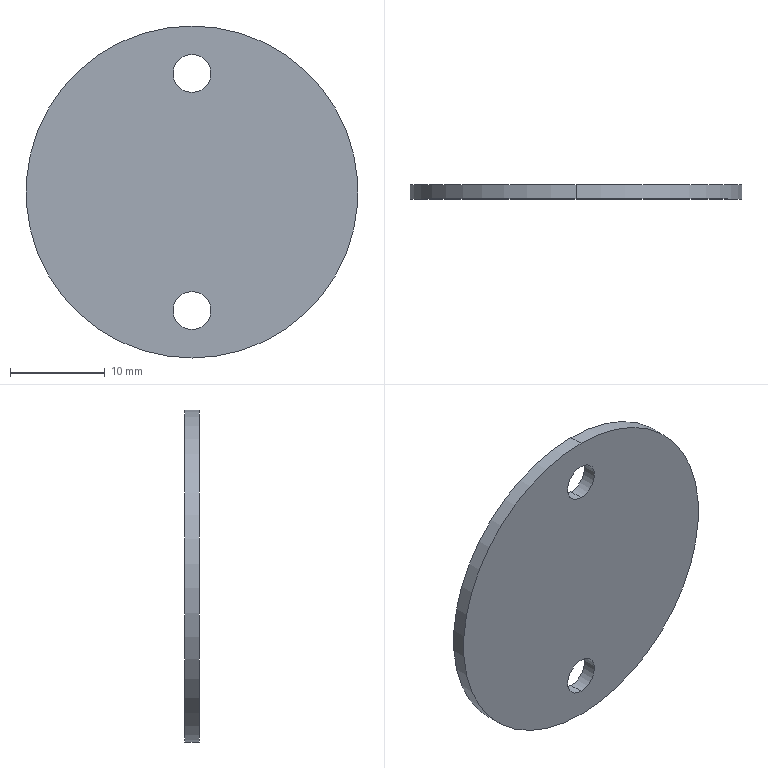Part | STEP file | 1519D1-4.stp.STEP | 1 solid | 8 faces | box 35 x 1.5 x 35 mm | volume 1405 mm3 | cylinder 6 | plane 2 | commonest cylinder face diameters 4 x4 35 x2
STEP:
#1=CARTESIAN_POINT('',(0.,0.,14.5));
#2=VERTEX_POINT('',#1);
#3=CARTESIAN_POINT('',(0.,0.,10.5));
#4=VERTEX_POINT('',#3);
#5=CARTESIAN_POINT('',(0.,0.,12.5));
#6=DIRECTION('',(0.,1.,0.));
#7=DIRECTION('',(0.,0.,1.));
#8=AXIS2_PLACEMENT_3D('',#5,#6,#7);
#9=CIRCLE('',#8,2.);
#10=EDGE_CURVE('',#2,#4,#9,.T.);
#11=ORIENTED_EDGE('',*,*,#10,.T.);
#12=CARTESIAN_POINT('',(0.,0.,12.5));
#13=DIRECTION('',(0.,1.,0.));
#14=DIRECTION('',(0.,0.,-1.));
#15=AXIS2_PLACEMENT_3D('',#12,#13,#14);
#16=CIRCLE('',#15,2.);
#17=EDGE_CURVE('',#4,#2,#16,.T.);
#18=ORIENTED_EDGE('',*,*,#17,.T.);
#19=EDGE_LOOP('',(#11,#18));
#20=FACE_BOUND('',#19,.T.);
#21=CARTESIAN_POINT('',(0.,0.,-10.5));
#22=VERTEX_POINT('',#21);
#23=CARTESIAN_POINT('',(0.,0.,-14.5));
#24=VERTEX_POINT('',#23);
#25=CARTESIAN_POINT('',(0.,0.,-12.5));
#26=DIRECTION('',(0.,1.,0.));
#27=DIRECTION('',(0.,0.,1.));
#28=AXIS2_PLACEMENT_3D('',#25,#26,#27);
#29=CIRCLE('',#28,2.);
#30=EDGE_CURVE('',#22,#24,#29,.T.);
#31=ORIENTED_EDGE('',*,*,#30,.T.);
#32=CARTESIAN_POINT('',(0.,0.,-12.5));
#33=DIRECTION('',(0.,1.,0.));
#34=DIRECTION('',(0.,0.,-1.));
#35=AXIS2_PLACEMENT_3D('',#32,#33,#34);
#36=CIRCLE('',#35,2.);
#37=EDGE_CURVE('',#24,#22,#36,.T.);
#38=ORIENTED_EDGE('',*,*,#37,.T.);
#39=EDGE_LOOP('',(#31,#38));
#40=FACE_BOUND('',#39,.T.);
#41=CARTESIAN_POINT('',(0.,0.,17.5));
#42=VERTEX_POINT('',#41);
#43=CARTESIAN_POINT('',(0.,0.,-17.5));
#44=VERTEX_POINT('',#43);
#45=CARTESIAN_POINT('',(0.,0.,0.));
#46=DIRECTION('',(0.,1.,0.));
#47=DIRECTION('',(0.,0.,1.));
#48=AXIS2_PLACEMENT_3D('',#45,#46,#47);
#49=CIRCLE('',#48,17.5);
#50=EDGE_CURVE('',#42,#44,#49,.T.);
#51=ORIENTED_EDGE('',*,*,#50,.F.);
#52=CARTESIAN_POINT('',(0.,0.,0.));
#53=DIRECTION('',(0.,1.,0.));
#54=DIRECTION('',(0.,0.,-1.));
#55=AXIS2_PLACEMENT_3D('',#52,#53,#54);
#56=CIRCLE('',#55,17.5);
#57=EDGE_CURVE('',#44,#42,#56,.T.);
#58=ORIENTED_EDGE('',*,*,#57,.F.);
#59=EDGE_LOOP('',(#51,#58));
#60=FACE_OUTER_BOUND('',#59,.T.);
#61=CARTESIAN_POINT('',(0.,0.,0.));
#62=DIRECTION('',(0.,1.,0.));
#63=DIRECTION('',(1.,0.,0.));
#64=AXIS2_PLACEMENT_3D('',#61,#62,#63);
#65=PLANE('',#64);
#66=ADVANCED_FACE('',(#20,#40,#60),#65,.F.);
#67=CARTESIAN_POINT('',(0.,1.5,17.5));
#68=VERTEX_POINT('',#67);
#69=CARTESIAN_POINT('',(0.,0.,17.5));
#70=DIRECTION('',(0.,1.,0.));
#71=VECTOR('',#70,1000.);
#72=LINE('',#69,#71);
#73=EDGE_CURVE('',#42,#68,#72,.T.);
#74=ORIENTED_EDGE('',*,*,#73,.T.);
#75=CARTESIAN_POINT('',(0.,1.5,-17.5));
#76=VERTEX_POINT('',#75);
#77=CARTESIAN_POINT('',(0.,1.5,0.));
#78=DIRECTION('',(0.,1.,0.));
#79=DIRECTION('',(0.,0.,-1.));
#80=AXIS2_PLACEMENT_3D('',#77,#78,#79);
#81=CIRCLE('',#80,17.5);
#82=EDGE_CURVE('',#76,#68,#81,.T.);
#83=ORIENTED_EDGE('',*,*,#82,.F.);
#84=CARTESIAN_POINT('',(0.,0.,-17.5));
#85=DIRECTION('',(0.,1.,0.));
#86=VECTOR('',#85,1000.);
#87=LINE('',#84,#86);
#88=EDGE_CURVE('',#44,#76,#87,.T.);
#89=ORIENTED_EDGE('',*,*,#88,.F.);
#90=ORIENTED_EDGE('',*,*,#57,.T.);
#91=EDGE_LOOP('',(#74,#83,#89,#90));
#92=FACE_OUTER_BOUND('',#91,.T.);
#93=CARTESIAN_POINT('',(0.,0.,0.));
#94=DIRECTION('',(0.,1.,0.));
#95=DIRECTION('',(0.,0.,-1.));
#96=AXIS2_PLACEMENT_3D('',#93,#94,#95);
#97=CYLINDRICAL_SURFACE('',#96,17.5);
#98=ADVANCED_FACE('',(#92),#97,.T.);
#99=ORIENTED_EDGE('',*,*,#88,.T.);
#100=CARTESIAN_POINT('',(0.,1.5,0.));
#101=DIRECTION('',(0.,1.,0.));
#102=DIRECTION('',(0.,0.,1.));
#103=AXIS2_PLACEMENT_3D('',#100,#101,#102);
#104=CIRCLE('',#103,17.5);
#105=EDGE_CURVE('',#68,#76,#104,.T.);
#106=ORIENTED_EDGE('',*,*,#105,.F.);
#107=ORIENTED_EDGE('',*,*,#73,.F.);
#108=ORIENTED_EDGE('',*,*,#50,.T.);
#109=EDGE_LOOP('',(#99,#106,#107,#108));
#110=FACE_OUTER_BOUND('',#109,.T.);
#111=CARTESIAN_POINT('',(0.,0.,0.));
#112=DIRECTION('',(0.,1.,0.));
#113=DIRECTION('',(0.,0.,-1.));
#114=AXIS2_PLACEMENT_3D('',#111,#112,#113);
#115=CYLINDRICAL_SURFACE('',#114,17.5);
#116=ADVANCED_FACE('',(#110),#115,.T.);
#117=CARTESIAN_POINT('',(0.,1.5,14.5));
#118=VERTEX_POINT('',#117);
#119=CARTESIAN_POINT('',(0.,1.5,10.5));
#120=VERTEX_POINT('',#119);
#121=CARTESIAN_POINT('',(0.,1.5,12.5));
#122=DIRECTION('',(0.,1.,0.));
#123=DIRECTION('',(0.,0.,1.));
#124=AXIS2_PLACEMENT_3D('',#121,#122,#123);
#125=CIRCLE('',#124,2.);
#126=EDGE_CURVE('',#118,#120,#125,.T.);
#127=ORIENTED_EDGE('',*,*,#126,.F.);
#128=CARTESIAN_POINT('',(0.,1.5,12.5));
#129=DIRECTION('',(0.,1.,0.));
#130=DIRECTION('',(0.,0.,-1.));
#131=AXIS2_PLACEMENT_3D('',#128,#129,#130);
#132=CIRCLE('',#131,2.);
#133=EDGE_CURVE('',#120,#118,#132,.T.);
#134=ORIENTED_EDGE('',*,*,#133,.F.);
#135=EDGE_LOOP('',(#127,#134));
#136=FACE_BOUND('',#135,.T.);
#137=CARTESIAN_POINT('',(0.,1.5,-10.5));
#138=VERTEX_POINT('',#137);
#139=CARTESIAN_POINT('',(0.,1.5,-14.5));
#140=VERTEX_POINT('',#139);
#141=CARTESIAN_POINT('',(0.,1.5,-12.5));
#142=DIRECTION('',(0.,1.,0.));
#143=DIRECTION('',(0.,0.,1.));
#144=AXIS2_PLACEMENT_3D('',#141,#142,#143);
#145=CIRCLE('',#144,2.);
#146=EDGE_CURVE('',#138,#140,#145,.T.);
#147=ORIENTED_EDGE('',*,*,#146,.F.);
#148=CARTESIAN_POINT('',(0.,1.5,-12.5));
#149=DIRECTION('',(0.,1.,0.));
#150=DIRECTION('',(0.,0.,-1.));
#151=AXIS2_PLACEMENT_3D('',#148,#149,#150);
#152=CIRCLE('',#151,2.);
#153=EDGE_CURVE('',#140,#138,#152,.T.);
#154=ORIENTED_EDGE('',*,*,#153,.F.);
#155=EDGE_LOOP('',(#147,#154));
#156=FACE_BOUND('',#155,.T.);
#157=ORIENTED_EDGE('',*,*,#105,.T.);
#158=ORIENTED_EDGE('',*,*,#82,.T.);
#159=EDGE_LOOP('',(#157,#158));
#160=FACE_OUTER_BOUND('',#159,.T.);
#161=CARTESIAN_POINT('',(0.,1.5,0.));
#162=DIRECTION('',(0.,1.,0.));
#163=DIRECTION('',(1.,0.,0.));
#164=AXIS2_PLACEMENT_3D('',#161,#162,#163);
#165=PLANE('',#164);
#166=ADVANCED_FACE('',(#136,#156,#160),#165,.T.);
#167=CARTESIAN_POINT('',(0.,1.5,10.5));
#168=DIRECTION('',(0.,-1.,0.));
#169=VECTOR('',#168,1000.);
#170=LINE('',#167,#169);
#171=EDGE_CURVE('',#120,#4,#170,.T.);
#172=ORIENTED_EDGE('',*,*,#171,.F.);
#173=ORIENTED_EDGE('',*,*,#133,.T.);
#174=CARTESIAN_POINT('',(0.,1.5,14.5));
#175=DIRECTION('',(0.,-1.,0.));
#176=VECTOR('',#175,1000.);
#177=LINE('',#174,#176);
#178=EDGE_CURVE('',#118,#2,#177,.T.);
#179=ORIENTED_EDGE('',*,*,#178,.T.);
#180=ORIENTED_EDGE('',*,*,#17,.F.);
#181=EDGE_LOOP('',(#172,#173,#179,#180));
#182=FACE_OUTER_BOUND('',#181,.T.);
#183=CARTESIAN_POINT('',(0.,1.5,12.5));
#184=DIRECTION('',(0.,1.,0.));
#185=DIRECTION('',(0.,0.,-1.));
#186=AXIS2_PLACEMENT_3D('',#183,#184,#185);
#187=CYLINDRICAL_SURFACE('',#186,2.);
#188=ADVANCED_FACE('',(#182),#187,.F.);
#189=ORIENTED_EDGE('',*,*,#178,.F.);
#190=ORIENTED_EDGE('',*,*,#126,.T.);
#191=ORIENTED_EDGE('',*,*,#171,.T.);
#192=ORIENTED_EDGE('',*,*,#10,.F.);
#193=EDGE_LOOP('',(#189,#190,#191,#192));
#194=FACE_OUTER_BOUND('',#193,.T.);
#195=CARTESIAN_POINT('',(0.,1.5,12.5));
#196=DIRECTION('',(0.,1.,0.));
#197=DIRECTION('',(0.,0.,-1.));
#198=AXIS2_PLACEMENT_3D('',#195,#196,#197);
#199=CYLINDRICAL_SURFACE('',#198,2.);
#200=ADVANCED_FACE('',(#194),#199,.F.);
#201=CARTESIAN_POINT('',(0.,1.5,-14.5));
#202=DIRECTION('',(0.,-1.,0.));
#203=VECTOR('',#202,1000.);
#204=LINE('',#201,#203);
#205=EDGE_CURVE('',#140,#24,#204,.T.);
#206=ORIENTED_EDGE('',*,*,#205,.F.);
#207=ORIENTED_EDGE('',*,*,#153,.T.);
#208=CARTESIAN_POINT('',(0.,1.5,-10.5));
#209=DIRECTION('',(0.,-1.,0.));
#210=VECTOR('',#209,1000.);
#211=LINE('',#208,#210);
#212=EDGE_CURVE('',#138,#22,#211,.T.);
#213=ORIENTED_EDGE('',*,*,#212,.T.);
#214=ORIENTED_EDGE('',*,*,#37,.F.);
#215=EDGE_LOOP('',(#206,#207,#213,#214));
#216=FACE_OUTER_BOUND('',#215,.T.);
#217=CARTESIAN_POINT('',(0.,1.5,-12.5));
#218=DIRECTION('',(0.,1.,0.));
#219=DIRECTION('',(0.,0.,-1.));
#220=AXIS2_PLACEMENT_3D('',#217,#218,#219);
#221=CYLINDRICAL_SURFACE('',#220,2.);
#222=ADVANCED_FACE('',(#216),#221,.F.);
#223=ORIENTED_EDGE('',*,*,#212,.F.);
#224=ORIENTED_EDGE('',*,*,#146,.T.);
#225=ORIENTED_EDGE('',*,*,#205,.T.);
#226=ORIENTED_EDGE('',*,*,#30,.F.);
#227=EDGE_LOOP('',(#223,#224,#225,#226));
#228=FACE_OUTER_BOUND('',#227,.T.);
#229=CARTESIAN_POINT('',(0.,1.5,-12.5));
#230=DIRECTION('',(0.,1.,0.));
#231=DIRECTION('',(0.,0.,-1.));
#232=AXIS2_PLACEMENT_3D('',#229,#230,#231);
#233=CYLINDRICAL_SURFACE('',#232,2.);
#234=ADVANCED_FACE('',(#228),#233,.F.);
#235=CLOSED_SHELL('',(#66,#98,#116,#166,#188,#200,#222,#234));
#236=MANIFOLD_SOLID_BREP('',#235);
#237=CARTESIAN_POINT('',(0.,0.,0.));
#238=DIRECTION('',(0.,0.,1.));
#239=DIRECTION('',(1.,0.,0.));
#240=AXIS2_PLACEMENT_3D('',#237,#238,#239);
#241=(LENGTH_UNIT()NAMED_UNIT(*)SI_UNIT(.MILLI.,.METRE.));
#242=UNCERTAINTY_MEASURE_WITH_UNIT(LENGTH_MEASURE(0.00001),#241,'','');
#243=(NAMED_UNIT(*)PLANE_ANGLE_UNIT()SI_UNIT($,.RADIAN.));
#244=(NAMED_UNIT(*)SI_UNIT($,.STERADIAN.)SOLID_ANGLE_UNIT());
#245=(GEOMETRIC_REPRESENTATION_CONTEXT(3)GLOBAL_UNCERTAINTY_ASSIGNED_CONTEXT((#242))GLOBAL_UNIT_ASSIGNED_CONTEXT((#241,#243,#244))REPRESENTATION_CONTEXT('',''));
#246=ADVANCED_BREP_SHAPE_REPRESENTATION('',(#236,#240),#245);